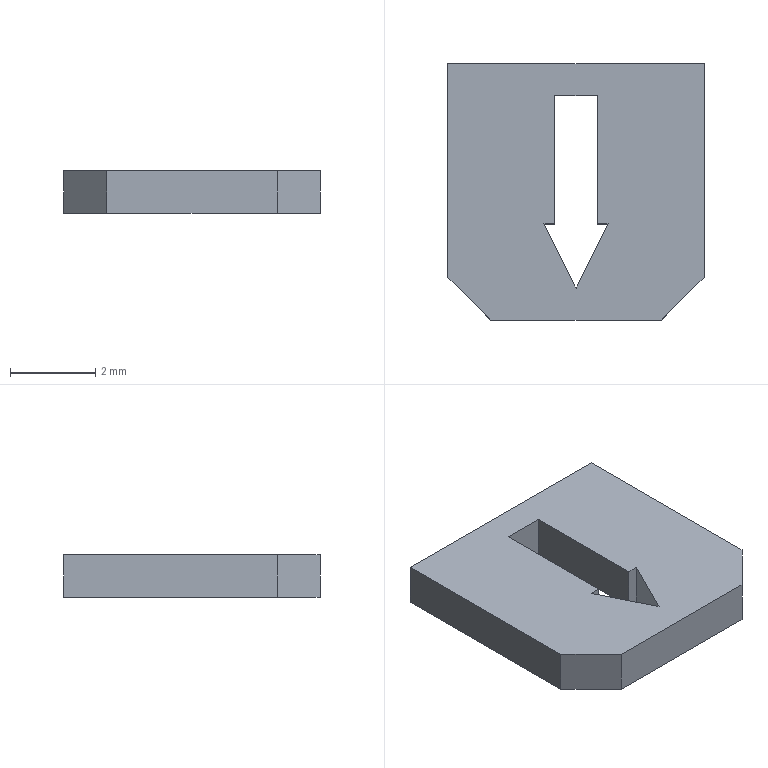Part | STEP file | OP-85138-Part-2-6 | 1 solid | 15 faces | box 6 x 6 x 1 mm | volume 30.875 mm3 | plane 15
STEP:
#1=CARTESIAN_POINT('',(3.75,2.25,0.));
#2=VERTEX_POINT('',#1);
#3=CARTESIAN_POINT('',(3.,0.75,0.));
#4=VERTEX_POINT('',#3);
#5=CARTESIAN_POINT('',(3.3,1.35,0.));
#6=DIRECTION('',(-0.4472,-0.8944,0.));
#7=VECTOR('',#6,1000.);
#8=LINE('',#5,#7);
#9=EDGE_CURVE('',#2,#4,#8,.T.);
#10=ORIENTED_EDGE('',*,*,#9,.F.);
#11=CARTESIAN_POINT('',(3.5,2.25,0.));
#12=VERTEX_POINT('',#11);
#13=CARTESIAN_POINT('',(3.,2.25,0.));
#14=DIRECTION('',(-1.,0.,0.));
#15=VECTOR('',#14,1000.);
#16=LINE('',#13,#15);
#17=EDGE_CURVE('',#2,#12,#16,.T.);
#18=ORIENTED_EDGE('',*,*,#17,.T.);
#19=CARTESIAN_POINT('',(3.5,5.25,0.));
#20=VERTEX_POINT('',#19);
#21=CARTESIAN_POINT('',(3.5,3.75,0.));
#22=DIRECTION('',(0.,1.,0.));
#23=VECTOR('',#22,1000.);
#24=LINE('',#21,#23);
#25=EDGE_CURVE('',#12,#20,#24,.T.);
#26=ORIENTED_EDGE('',*,*,#25,.T.);
#27=CARTESIAN_POINT('',(2.5,5.25,0.));
#28=VERTEX_POINT('',#27);
#29=CARTESIAN_POINT('',(3.,5.25,0.));
#30=DIRECTION('',(-1.,0.,0.));
#31=VECTOR('',#30,1000.);
#32=LINE('',#29,#31);
#33=EDGE_CURVE('',#20,#28,#32,.T.);
#34=ORIENTED_EDGE('',*,*,#33,.T.);
#35=CARTESIAN_POINT('',(2.5,2.25,0.));
#36=VERTEX_POINT('',#35);
#37=CARTESIAN_POINT('',(2.5,3.75,0.));
#38=DIRECTION('',(0.,-1.,0.));
#39=VECTOR('',#38,1000.);
#40=LINE('',#37,#39);
#41=EDGE_CURVE('',#28,#36,#40,.T.);
#42=ORIENTED_EDGE('',*,*,#41,.T.);
#43=CARTESIAN_POINT('',(2.25,2.25,0.));
#44=VERTEX_POINT('',#43);
#45=CARTESIAN_POINT('',(3.,2.25,0.));
#46=DIRECTION('',(-1.,0.,0.));
#47=VECTOR('',#46,1000.);
#48=LINE('',#45,#47);
#49=EDGE_CURVE('',#36,#44,#48,.T.);
#50=ORIENTED_EDGE('',*,*,#49,.T.);
#51=CARTESIAN_POINT('',(2.7,1.35,0.));
#52=DIRECTION('',(-0.4472,0.8944,0.));
#53=VECTOR('',#52,1000.);
#54=LINE('',#51,#53);
#55=EDGE_CURVE('',#4,#44,#54,.T.);
#56=ORIENTED_EDGE('',*,*,#55,.F.);
#57=EDGE_LOOP('',(#10,#18,#26,#34,#42,#50,#56));
#58=FACE_BOUND('',#57,.T.);
#59=CARTESIAN_POINT('',(1.,0.,0.));
#60=VERTEX_POINT('',#59);
#61=CARTESIAN_POINT('',(5.,0.,0.));
#62=VERTEX_POINT('',#61);
#63=CARTESIAN_POINT('',(3.,0.,0.));
#64=DIRECTION('',(1.,0.,0.));
#65=VECTOR('',#64,1000.);
#66=LINE('',#63,#65);
#67=EDGE_CURVE('',#60,#62,#66,.T.);
#68=ORIENTED_EDGE('',*,*,#67,.F.);
#69=CARTESIAN_POINT('',(0.,1.,0.));
#70=VERTEX_POINT('',#69);
#71=CARTESIAN_POINT('',(0.5,0.5,0.));
#72=DIRECTION('',(-0.7071,0.7071,0.));
#73=VECTOR('',#72,1000.);
#74=LINE('',#71,#73);
#75=EDGE_CURVE('',#60,#70,#74,.T.);
#76=ORIENTED_EDGE('',*,*,#75,.T.);
#77=CARTESIAN_POINT('',(0.,6.,0.));
#78=VERTEX_POINT('',#77);
#79=CARTESIAN_POINT('',(0.,3.,0.));
#80=DIRECTION('',(0.,-1.,0.));
#81=VECTOR('',#80,1000.);
#82=LINE('',#79,#81);
#83=EDGE_CURVE('',#78,#70,#82,.T.);
#84=ORIENTED_EDGE('',*,*,#83,.F.);
#85=CARTESIAN_POINT('',(6.,6.,0.));
#86=VERTEX_POINT('',#85);
#87=CARTESIAN_POINT('',(3.,6.,0.));
#88=DIRECTION('',(-1.,0.,0.));
#89=VECTOR('',#88,1000.);
#90=LINE('',#87,#89);
#91=EDGE_CURVE('',#86,#78,#90,.T.);
#92=ORIENTED_EDGE('',*,*,#91,.F.);
#93=CARTESIAN_POINT('',(6.,1.,0.));
#94=VERTEX_POINT('',#93);
#95=CARTESIAN_POINT('',(6.,3.,0.));
#96=DIRECTION('',(0.,1.,0.));
#97=VECTOR('',#96,1000.);
#98=LINE('',#95,#97);
#99=EDGE_CURVE('',#94,#86,#98,.T.);
#100=ORIENTED_EDGE('',*,*,#99,.F.);
#101=CARTESIAN_POINT('',(5.5,0.5,0.));
#102=DIRECTION('',(-0.7071,-0.7071,0.));
#103=VECTOR('',#102,1000.);
#104=LINE('',#101,#103);
#105=EDGE_CURVE('',#94,#62,#104,.T.);
#106=ORIENTED_EDGE('',*,*,#105,.T.);
#107=EDGE_LOOP('',(#68,#76,#84,#92,#100,#106));
#108=FACE_OUTER_BOUND('',#107,.T.);
#109=CARTESIAN_POINT('',(3.,3.,0.));
#110=DIRECTION('',(0.,0.,-1.));
#111=DIRECTION('',(1.,0.,0.));
#112=AXIS2_PLACEMENT_3D('',#109,#110,#111);
#113=PLANE('',#112);
#114=ADVANCED_FACE('',(#58,#108),#113,.T.);
#115=CARTESIAN_POINT('',(6.,6.,1.));
#116=VERTEX_POINT('',#115);
#117=CARTESIAN_POINT('',(6.,6.,1.));
#118=DIRECTION('',(0.,0.,-1.));
#119=VECTOR('',#118,1000.);
#120=LINE('',#117,#119);
#121=EDGE_CURVE('',#116,#86,#120,.T.);
#122=ORIENTED_EDGE('',*,*,#121,.T.);
#123=ORIENTED_EDGE('',*,*,#91,.T.);
#124=CARTESIAN_POINT('',(0.,6.,1.));
#125=VERTEX_POINT('',#124);
#126=CARTESIAN_POINT('',(0.,6.,1.));
#127=DIRECTION('',(0.,0.,-1.));
#128=VECTOR('',#127,1000.);
#129=LINE('',#126,#128);
#130=EDGE_CURVE('',#125,#78,#129,.T.);
#131=ORIENTED_EDGE('',*,*,#130,.F.);
#132=CARTESIAN_POINT('',(3.,6.,1.));
#133=DIRECTION('',(1.,0.,0.));
#134=VECTOR('',#133,1000.);
#135=LINE('',#132,#134);
#136=EDGE_CURVE('',#125,#116,#135,.T.);
#137=ORIENTED_EDGE('',*,*,#136,.T.);
#138=EDGE_LOOP('',(#122,#123,#131,#137));
#139=FACE_OUTER_BOUND('',#138,.T.);
#140=CARTESIAN_POINT('',(3.,6.,1.));
#141=DIRECTION('',(0.,1.,0.));
#142=DIRECTION('',(0.,0.,1.));
#143=AXIS2_PLACEMENT_3D('',#140,#141,#142);
#144=PLANE('',#143);
#145=ADVANCED_FACE('',(#139),#144,.T.);
#146=ORIENTED_EDGE('',*,*,#83,.T.);
#147=CARTESIAN_POINT('',(0.,1.,1.));
#148=VERTEX_POINT('',#147);
#149=CARTESIAN_POINT('',(0.,1.,1.));
#150=DIRECTION('',(0.,0.,1.));
#151=VECTOR('',#150,1000.);
#152=LINE('',#149,#151);
#153=EDGE_CURVE('',#70,#148,#152,.T.);
#154=ORIENTED_EDGE('',*,*,#153,.T.);
#155=CARTESIAN_POINT('',(0.,3.,1.));
#156=DIRECTION('',(0.,1.,0.));
#157=VECTOR('',#156,1000.);
#158=LINE('',#155,#157);
#159=EDGE_CURVE('',#148,#125,#158,.T.);
#160=ORIENTED_EDGE('',*,*,#159,.T.);
#161=ORIENTED_EDGE('',*,*,#130,.T.);
#162=EDGE_LOOP('',(#146,#154,#160,#161));
#163=FACE_OUTER_BOUND('',#162,.T.);
#164=CARTESIAN_POINT('',(0.,3.,1.));
#165=DIRECTION('',(-1.,0.,0.));
#166=DIRECTION('',(0.,0.,-1.));
#167=AXIS2_PLACEMENT_3D('',#164,#165,#166);
#168=PLANE('',#167);
#169=ADVANCED_FACE('',(#163),#168,.T.);
#170=CARTESIAN_POINT('',(5.,0.,1.));
#171=VERTEX_POINT('',#170);
#172=CARTESIAN_POINT('',(1.,0.,1.));
#173=VERTEX_POINT('',#172);
#174=CARTESIAN_POINT('',(3.,0.,1.));
#175=DIRECTION('',(-1.,0.,0.));
#176=VECTOR('',#175,1000.);
#177=LINE('',#174,#176);
#178=EDGE_CURVE('',#171,#173,#177,.T.);
#179=ORIENTED_EDGE('',*,*,#178,.T.);
#180=CARTESIAN_POINT('',(1.,0.,1.));
#181=DIRECTION('',(0.,0.,-1.));
#182=VECTOR('',#181,1000.);
#183=LINE('',#180,#182);
#184=EDGE_CURVE('',#173,#60,#183,.T.);
#185=ORIENTED_EDGE('',*,*,#184,.T.);
#186=ORIENTED_EDGE('',*,*,#67,.T.);
#187=CARTESIAN_POINT('',(5.,0.,1.));
#188=DIRECTION('',(0.,0.,1.));
#189=VECTOR('',#188,1000.);
#190=LINE('',#187,#189);
#191=EDGE_CURVE('',#62,#171,#190,.T.);
#192=ORIENTED_EDGE('',*,*,#191,.T.);
#193=EDGE_LOOP('',(#179,#185,#186,#192));
#194=FACE_OUTER_BOUND('',#193,.T.);
#195=CARTESIAN_POINT('',(3.,0.,1.));
#196=DIRECTION('',(0.,-1.,0.));
#197=DIRECTION('',(0.,0.,-1.));
#198=AXIS2_PLACEMENT_3D('',#195,#196,#197);
#199=PLANE('',#198);
#200=ADVANCED_FACE('',(#194),#199,.T.);
#201=CARTESIAN_POINT('',(3.,0.75,1.));
#202=VERTEX_POINT('',#201);
#203=CARTESIAN_POINT('',(3.75,2.25,1.));
#204=VERTEX_POINT('',#203);
#205=CARTESIAN_POINT('',(3.3,1.35,1.));
#206=DIRECTION('',(0.4472,0.8944,0.));
#207=VECTOR('',#206,1000.);
#208=LINE('',#205,#207);
#209=EDGE_CURVE('',#202,#204,#208,.T.);
#210=ORIENTED_EDGE('',*,*,#209,.F.);
#211=CARTESIAN_POINT('',(2.25,2.25,1.));
#212=VERTEX_POINT('',#211);
#213=CARTESIAN_POINT('',(2.7,1.35,1.));
#214=DIRECTION('',(0.4472,-0.8944,0.));
#215=VECTOR('',#214,1000.);
#216=LINE('',#213,#215);
#217=EDGE_CURVE('',#212,#202,#216,.T.);
#218=ORIENTED_EDGE('',*,*,#217,.F.);
#219=CARTESIAN_POINT('',(2.5,2.25,1.));
#220=VERTEX_POINT('',#219);
#221=CARTESIAN_POINT('',(3.,2.25,1.));
#222=DIRECTION('',(1.,0.,0.));
#223=VECTOR('',#222,1000.);
#224=LINE('',#221,#223);
#225=EDGE_CURVE('',#212,#220,#224,.T.);
#226=ORIENTED_EDGE('',*,*,#225,.T.);
#227=CARTESIAN_POINT('',(2.5,5.25,1.));
#228=VERTEX_POINT('',#227);
#229=CARTESIAN_POINT('',(2.5,3.75,1.));
#230=DIRECTION('',(0.,1.,0.));
#231=VECTOR('',#230,1000.);
#232=LINE('',#229,#231);
#233=EDGE_CURVE('',#220,#228,#232,.T.);
#234=ORIENTED_EDGE('',*,*,#233,.T.);
#235=CARTESIAN_POINT('',(3.5,5.25,1.));
#236=VERTEX_POINT('',#235);
#237=CARTESIAN_POINT('',(3.,5.25,1.));
#238=DIRECTION('',(1.,0.,0.));
#239=VECTOR('',#238,1000.);
#240=LINE('',#237,#239);
#241=EDGE_CURVE('',#228,#236,#240,.T.);
#242=ORIENTED_EDGE('',*,*,#241,.T.);
#243=CARTESIAN_POINT('',(3.5,2.25,1.));
#244=VERTEX_POINT('',#243);
#245=CARTESIAN_POINT('',(3.5,3.75,1.));
#246=DIRECTION('',(0.,-1.,0.));
#247=VECTOR('',#246,1000.);
#248=LINE('',#245,#247);
#249=EDGE_CURVE('',#236,#244,#248,.T.);
#250=ORIENTED_EDGE('',*,*,#249,.T.);
#251=CARTESIAN_POINT('',(3.,2.25,1.));
#252=DIRECTION('',(1.,0.,0.));
#253=VECTOR('',#252,1000.);
#254=LINE('',#251,#253);
#255=EDGE_CURVE('',#244,#204,#254,.T.);
#256=ORIENTED_EDGE('',*,*,#255,.T.);
#257=EDGE_LOOP('',(#210,#218,#226,#234,#242,#250,#256));
#258=FACE_BOUND('',#257,.T.);
#259=ORIENTED_EDGE('',*,*,#159,.F.);
#260=CARTESIAN_POINT('',(0.5,0.5,1.));
#261=DIRECTION('',(0.7071,-0.7071,0.));
#262=VECTOR('',#261,1000.);
#263=LINE('',#260,#262);
#264=EDGE_CURVE('',#148,#173,#263,.T.);
#265=ORIENTED_EDGE('',*,*,#264,.T.);
#266=ORIENTED_EDGE('',*,*,#178,.F.);
#267=CARTESIAN_POINT('',(6.,1.,1.));
#268=VERTEX_POINT('',#267);
#269=CARTESIAN_POINT('',(5.5,0.5,1.));
#270=DIRECTION('',(0.7071,0.7071,0.));
#271=VECTOR('',#270,1000.);
#272=LINE('',#269,#271);
#273=EDGE_CURVE('',#171,#268,#272,.T.);
#274=ORIENTED_EDGE('',*,*,#273,.T.);
#275=CARTESIAN_POINT('',(6.,3.,1.));
#276=DIRECTION('',(0.,-1.,0.));
#277=VECTOR('',#276,1000.);
#278=LINE('',#275,#277);
#279=EDGE_CURVE('',#116,#268,#278,.T.);
#280=ORIENTED_EDGE('',*,*,#279,.F.);
#281=ORIENTED_EDGE('',*,*,#136,.F.);
#282=EDGE_LOOP('',(#259,#265,#266,#274,#280,#281));
#283=FACE_OUTER_BOUND('',#282,.T.);
#284=CARTESIAN_POINT('',(3.,3.,1.));
#285=DIRECTION('',(0.,0.,1.));
#286=DIRECTION('',(-1.,0.,0.));
#287=AXIS2_PLACEMENT_3D('',#284,#285,#286);
#288=PLANE('',#287);
#289=ADVANCED_FACE('',(#258,#283),#288,.T.);
#290=ORIENTED_EDGE('',*,*,#279,.T.);
#291=CARTESIAN_POINT('',(6.,1.,1.));
#292=DIRECTION('',(0.,0.,-1.));
#293=VECTOR('',#292,1000.);
#294=LINE('',#291,#293);
#295=EDGE_CURVE('',#268,#94,#294,.T.);
#296=ORIENTED_EDGE('',*,*,#295,.T.);
#297=ORIENTED_EDGE('',*,*,#99,.T.);
#298=ORIENTED_EDGE('',*,*,#121,.F.);
#299=EDGE_LOOP('',(#290,#296,#297,#298));
#300=FACE_OUTER_BOUND('',#299,.T.);
#301=CARTESIAN_POINT('',(6.,3.,1.));
#302=DIRECTION('',(1.,0.,0.));
#303=DIRECTION('',(0.,0.,1.));
#304=AXIS2_PLACEMENT_3D('',#301,#302,#303);
#305=PLANE('',#304);
#306=ADVANCED_FACE('',(#300),#305,.T.);
#307=ORIENTED_EDGE('',*,*,#273,.F.);
#308=ORIENTED_EDGE('',*,*,#191,.F.);
#309=ORIENTED_EDGE('',*,*,#105,.F.);
#310=ORIENTED_EDGE('',*,*,#295,.F.);
#311=EDGE_LOOP('',(#307,#308,#309,#310));
#312=FACE_OUTER_BOUND('',#311,.T.);
#313=CARTESIAN_POINT('',(6.,1.,1.));
#314=DIRECTION('',(-0.7071,0.7071,0.));
#315=DIRECTION('',(0.,0.,-1.));
#316=AXIS2_PLACEMENT_3D('',#313,#314,#315);
#317=PLANE('',#316);
#318=ADVANCED_FACE('',(#312),#317,.F.);
#319=ORIENTED_EDGE('',*,*,#264,.F.);
#320=ORIENTED_EDGE('',*,*,#153,.F.);
#321=ORIENTED_EDGE('',*,*,#75,.F.);
#322=ORIENTED_EDGE('',*,*,#184,.F.);
#323=EDGE_LOOP('',(#319,#320,#321,#322));
#324=FACE_OUTER_BOUND('',#323,.T.);
#325=CARTESIAN_POINT('',(1.,0.,1.));
#326=DIRECTION('',(0.7071,0.7071,0.));
#327=DIRECTION('',(0.,0.,-1.));
#328=AXIS2_PLACEMENT_3D('',#325,#326,#327);
#329=PLANE('',#328);
#330=ADVANCED_FACE('',(#324),#329,.F.);
#331=ORIENTED_EDGE('',*,*,#17,.F.);
#332=CARTESIAN_POINT('',(3.75,2.25,0.));
#333=DIRECTION('',(0.,0.,1.));
#334=VECTOR('',#333,1000.);
#335=LINE('',#332,#334);
#336=EDGE_CURVE('',#2,#204,#335,.T.);
#337=ORIENTED_EDGE('',*,*,#336,.T.);
#338=ORIENTED_EDGE('',*,*,#255,.F.);
#339=CARTESIAN_POINT('',(3.5,2.25,0.));
#340=DIRECTION('',(0.,0.,1.));
#341=VECTOR('',#340,1000.);
#342=LINE('',#339,#341);
#343=EDGE_CURVE('',#12,#244,#342,.T.);
#344=ORIENTED_EDGE('',*,*,#343,.F.);
#345=EDGE_LOOP('',(#331,#337,#338,#344));
#346=FACE_OUTER_BOUND('',#345,.T.);
#347=CARTESIAN_POINT('',(3.,2.25,0.));
#348=DIRECTION('',(0.,1.,0.));
#349=DIRECTION('',(0.,0.,-1.));
#350=AXIS2_PLACEMENT_3D('',#347,#348,#349);
#351=PLANE('',#350);
#352=ADVANCED_FACE('',(#346),#351,.F.);
#353=CARTESIAN_POINT('',(2.5,2.25,0.));
#354=DIRECTION('',(0.,0.,1.));
#355=VECTOR('',#354,1000.);
#356=LINE('',#353,#355);
#357=EDGE_CURVE('',#36,#220,#356,.T.);
#358=ORIENTED_EDGE('',*,*,#357,.T.);
#359=ORIENTED_EDGE('',*,*,#225,.F.);
#360=CARTESIAN_POINT('',(2.25,2.25,0.));
#361=DIRECTION('',(0.,0.,1.));
#362=VECTOR('',#361,1000.);
#363=LINE('',#360,#362);
#364=EDGE_CURVE('',#44,#212,#363,.T.);
#365=ORIENTED_EDGE('',*,*,#364,.F.);
#366=ORIENTED_EDGE('',*,*,#49,.F.);
#367=EDGE_LOOP('',(#358,#359,#365,#366));
#368=FACE_OUTER_BOUND('',#367,.T.);
#369=CARTESIAN_POINT('',(3.,2.25,0.));
#370=DIRECTION('',(0.,1.,0.));
#371=DIRECTION('',(0.,0.,-1.));
#372=AXIS2_PLACEMENT_3D('',#369,#370,#371);
#373=PLANE('',#372);
#374=ADVANCED_FACE('',(#368),#373,.F.);
#375=ORIENTED_EDGE('',*,*,#9,.T.);
#376=CARTESIAN_POINT('',(3.,0.75,0.));
#377=DIRECTION('',(0.,0.,1.));
#378=VECTOR('',#377,1000.);
#379=LINE('',#376,#378);
#380=EDGE_CURVE('',#4,#202,#379,.T.);
#381=ORIENTED_EDGE('',*,*,#380,.T.);
#382=ORIENTED_EDGE('',*,*,#209,.T.);
#383=ORIENTED_EDGE('',*,*,#336,.F.);
#384=EDGE_LOOP('',(#375,#381,#382,#383));
#385=FACE_OUTER_BOUND('',#384,.T.);
#386=CARTESIAN_POINT('',(3.,0.75,0.));
#387=DIRECTION('',(-0.8944,0.4472,0.));
#388=DIRECTION('',(0.,0.,1.));
#389=AXIS2_PLACEMENT_3D('',#386,#387,#388);
#390=PLANE('',#389);
#391=ADVANCED_FACE('',(#385),#390,.T.);
#392=ORIENTED_EDGE('',*,*,#55,.T.);
#393=ORIENTED_EDGE('',*,*,#364,.T.);
#394=ORIENTED_EDGE('',*,*,#217,.T.);
#395=ORIENTED_EDGE('',*,*,#380,.F.);
#396=EDGE_LOOP('',(#392,#393,#394,#395));
#397=FACE_OUTER_BOUND('',#396,.T.);
#398=CARTESIAN_POINT('',(2.25,2.25,0.));
#399=DIRECTION('',(0.8944,0.4472,0.));
#400=DIRECTION('',(0.,0.,1.));
#401=AXIS2_PLACEMENT_3D('',#398,#399,#400);
#402=PLANE('',#401);
#403=ADVANCED_FACE('',(#397),#402,.T.);
#404=CARTESIAN_POINT('',(3.5,5.25,0.));
#405=DIRECTION('',(0.,0.,1.));
#406=VECTOR('',#405,1000.);
#407=LINE('',#404,#406);
#408=EDGE_CURVE('',#20,#236,#407,.T.);
#409=ORIENTED_EDGE('',*,*,#408,.F.);
#410=ORIENTED_EDGE('',*,*,#25,.F.);
#411=ORIENTED_EDGE('',*,*,#343,.T.);
#412=ORIENTED_EDGE('',*,*,#249,.F.);
#413=EDGE_LOOP('',(#409,#410,#411,#412));
#414=FACE_OUTER_BOUND('',#413,.T.);
#415=CARTESIAN_POINT('',(3.5,3.75,0.));
#416=DIRECTION('',(1.,0.,0.));
#417=DIRECTION('',(0.,0.,-1.));
#418=AXIS2_PLACEMENT_3D('',#415,#416,#417);
#419=PLANE('',#418);
#420=ADVANCED_FACE('',(#414),#419,.F.);
#421=ORIENTED_EDGE('',*,*,#357,.F.);
#422=ORIENTED_EDGE('',*,*,#41,.F.);
#423=CARTESIAN_POINT('',(2.5,5.25,0.));
#424=DIRECTION('',(0.,0.,1.));
#425=VECTOR('',#424,1000.);
#426=LINE('',#423,#425);
#427=EDGE_CURVE('',#28,#228,#426,.T.);
#428=ORIENTED_EDGE('',*,*,#427,.T.);
#429=ORIENTED_EDGE('',*,*,#233,.F.);
#430=EDGE_LOOP('',(#421,#422,#428,#429));
#431=FACE_OUTER_BOUND('',#430,.T.);
#432=CARTESIAN_POINT('',(2.5,3.75,0.));
#433=DIRECTION('',(-1.,0.,0.));
#434=DIRECTION('',(0.,0.,1.));
#435=AXIS2_PLACEMENT_3D('',#432,#433,#434);
#436=PLANE('',#435);
#437=ADVANCED_FACE('',(#431),#436,.F.);
#438=ORIENTED_EDGE('',*,*,#33,.F.);
#439=ORIENTED_EDGE('',*,*,#408,.T.);
#440=ORIENTED_EDGE('',*,*,#241,.F.);
#441=ORIENTED_EDGE('',*,*,#427,.F.);
#442=EDGE_LOOP('',(#438,#439,#440,#441));
#443=FACE_OUTER_BOUND('',#442,.T.);
#444=CARTESIAN_POINT('',(3.,5.25,0.));
#445=DIRECTION('',(0.,1.,0.));
#446=DIRECTION('',(0.,0.,-1.));
#447=AXIS2_PLACEMENT_3D('',#444,#445,#446);
#448=PLANE('',#447);
#449=ADVANCED_FACE('',(#443),#448,.F.);
#450=CLOSED_SHELL('',(#114,#145,#169,#200,#289,#306,#318,#330,#352,#374,#391,#403,#420,#437,#449));
#451=MANIFOLD_SOLID_BREP('',#450);
#452=CARTESIAN_POINT('',(0.,0.,0.));
#453=DIRECTION('',(0.,0.,1.));
#454=DIRECTION('',(1.,0.,0.));
#455=AXIS2_PLACEMENT_3D('',#452,#453,#454);
#456=(LENGTH_UNIT()NAMED_UNIT(*)SI_UNIT(.MILLI.,.METRE.));
#457=UNCERTAINTY_MEASURE_WITH_UNIT(LENGTH_MEASURE(0.00001),#456,'','');
#458=(NAMED_UNIT(*)PLANE_ANGLE_UNIT()SI_UNIT($,.RADIAN.));
#459=(NAMED_UNIT(*)SI_UNIT($,.STERADIAN.)SOLID_ANGLE_UNIT());
#460=(GEOMETRIC_REPRESENTATION_CONTEXT(3)GLOBAL_UNCERTAINTY_ASSIGNED_CONTEXT((#457))GLOBAL_UNIT_ASSIGNED_CONTEXT((#456,#458,#459))REPRESENTATION_CONTEXT('',''));
#461=ADVANCED_BREP_SHAPE_REPRESENTATION('',(#451,#455),#460);